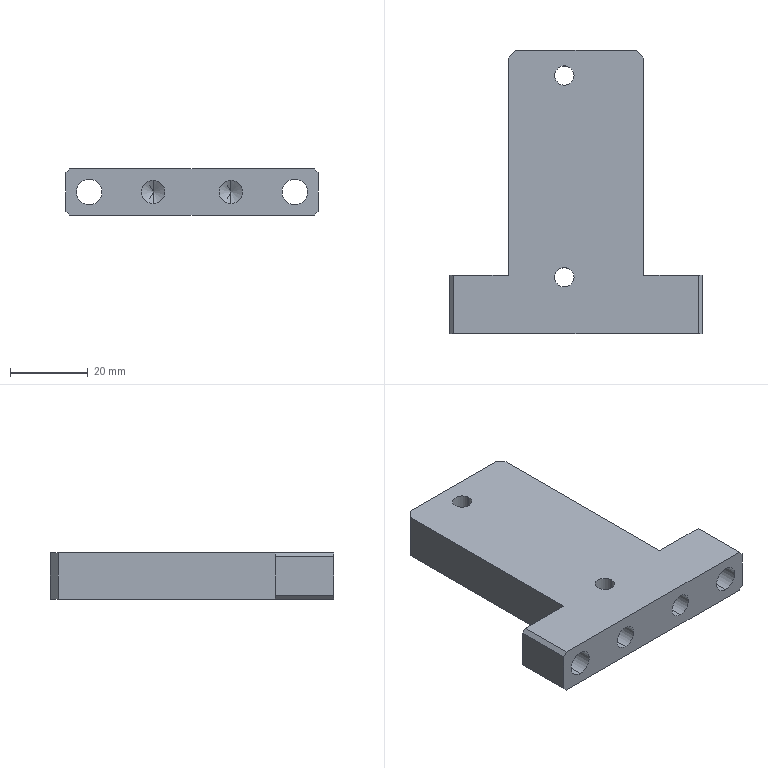Part | SolidWorks | features HoleWzd 3, Chamfer 2, Extrusion 1, ICE 1 | 1 solid | 32 faces | box 65 x 73 x 12 mm | volume 33602 mm3 | plane 16 | cylinder 12 | cone 4 | commonest cylinder face diameters 5 x4 6 x4 6.6 x4
STEP:
#1=CARTESIAN_POINT('',(-0.5,-22.,6.));
#2=VERTEX_POINT('',#1);
#3=CARTESIAN_POINT('',(-5.5,-22.,6.));
#4=VERTEX_POINT('',#3);
#5=CARTESIAN_POINT('',(-3.,-22.,6.));
#6=DIRECTION('',(0.,0.,-1.));
#7=DIRECTION('',(-1.,0.,0.));
#8=AXIS2_PLACEMENT_3D('',#5,#6,#7);
#9=CIRCLE('',#8,2.5);
#10=EDGE_CURVE('',#2,#4,#9,.T.);
#11=ORIENTED_EDGE('',*,*,#10,.F.);
#12=CARTESIAN_POINT('',(-0.5,-22.,-6.));
#13=VERTEX_POINT('',#12);
#14=CARTESIAN_POINT('',(-0.5,-22.,-6.));
#15=DIRECTION('',(0.,0.,-1.));
#16=VECTOR('',#15,1000.);
#17=LINE('',#14,#16);
#18=EDGE_CURVE('',#2,#13,#17,.T.);
#19=ORIENTED_EDGE('',*,*,#18,.T.);
#20=CARTESIAN_POINT('',(-5.5,-22.,-6.));
#21=VERTEX_POINT('',#20);
#22=CARTESIAN_POINT('',(-3.,-22.,-6.));
#23=DIRECTION('',(0.,0.,-1.));
#24=DIRECTION('',(-1.,0.,0.));
#25=AXIS2_PLACEMENT_3D('',#22,#23,#24);
#26=CIRCLE('',#25,2.5);
#27=EDGE_CURVE('',#13,#21,#26,.T.);
#28=ORIENTED_EDGE('',*,*,#27,.T.);
#29=CARTESIAN_POINT('',(-5.5,-22.,-6.));
#30=DIRECTION('',(0.,0.,-1.));
#31=VECTOR('',#30,1000.);
#32=LINE('',#29,#31);
#33=EDGE_CURVE('',#4,#21,#32,.T.);
#34=ORIENTED_EDGE('',*,*,#33,.F.);
#35=EDGE_LOOP('',(#11,#19,#28,#34));
#36=FACE_OUTER_BOUND('',#35,.T.);
#37=CARTESIAN_POINT('',(-3.,-22.,-6.));
#38=DIRECTION('',(0.,0.,-1.));
#39=DIRECTION('',(-1.,0.,0.));
#40=AXIS2_PLACEMENT_3D('',#37,#38,#39);
#41=CYLINDRICAL_SURFACE('',#40,2.5);
#42=ADVANCED_FACE('',(#36),#41,.F.);
#43=CARTESIAN_POINT('',(-0.5,30.,6.));
#44=VERTEX_POINT('',#43);
#45=CARTESIAN_POINT('',(-5.5,30.,6.));
#46=VERTEX_POINT('',#45);
#47=CARTESIAN_POINT('',(-3.,30.,6.));
#48=DIRECTION('',(0.,0.,-1.));
#49=DIRECTION('',(-1.,0.,0.));
#50=AXIS2_PLACEMENT_3D('',#47,#48,#49);
#51=CIRCLE('',#50,2.5);
#52=EDGE_CURVE('',#44,#46,#51,.T.);
#53=ORIENTED_EDGE('',*,*,#52,.F.);
#54=CARTESIAN_POINT('',(-0.5,30.,-6.));
#55=VERTEX_POINT('',#54);
#56=CARTESIAN_POINT('',(-0.5,30.,-6.));
#57=DIRECTION('',(0.,0.,-1.));
#58=VECTOR('',#57,1000.);
#59=LINE('',#56,#58);
#60=EDGE_CURVE('',#44,#55,#59,.T.);
#61=ORIENTED_EDGE('',*,*,#60,.T.);
#62=CARTESIAN_POINT('',(-5.5,30.,-6.));
#63=VERTEX_POINT('',#62);
#64=CARTESIAN_POINT('',(-3.,30.,-6.));
#65=DIRECTION('',(0.,0.,-1.));
#66=DIRECTION('',(-1.,0.,0.));
#67=AXIS2_PLACEMENT_3D('',#64,#65,#66);
#68=CIRCLE('',#67,2.5);
#69=EDGE_CURVE('',#55,#63,#68,.T.);
#70=ORIENTED_EDGE('',*,*,#69,.T.);
#71=CARTESIAN_POINT('',(-5.5,30.,-6.));
#72=DIRECTION('',(0.,0.,-1.));
#73=VECTOR('',#72,1000.);
#74=LINE('',#71,#73);
#75=EDGE_CURVE('',#46,#63,#74,.T.);
#76=ORIENTED_EDGE('',*,*,#75,.F.);
#77=EDGE_LOOP('',(#53,#61,#70,#76));
#78=FACE_OUTER_BOUND('',#77,.T.);
#79=CARTESIAN_POINT('',(-3.,30.,-6.));
#80=DIRECTION('',(0.,0.,-1.));
#81=DIRECTION('',(-1.,0.,0.));
#82=AXIS2_PLACEMENT_3D('',#79,#80,#81);
#83=CYLINDRICAL_SURFACE('',#82,2.5);
#84=ADVANCED_FACE('',(#78),#83,.F.);
#85=CARTESIAN_POINT('',(-10.,-21.5,3.));
#86=VERTEX_POINT('',#85);
#87=CARTESIAN_POINT('',(-10.,-21.5,-3.));
#88=VERTEX_POINT('',#87);
#89=CARTESIAN_POINT('',(-10.,-21.5,0.));
#90=DIRECTION('',(0.,-1.,0.));
#91=DIRECTION('',(0.,0.,-1.));
#92=AXIS2_PLACEMENT_3D('',#89,#90,#91);
#93=CIRCLE('',#92,3.);
#94=EDGE_CURVE('',#86,#88,#93,.T.);
#95=ORIENTED_EDGE('',*,*,#94,.F.);
#96=CARTESIAN_POINT('',(-10.,-36.5,3.));
#97=VERTEX_POINT('',#96);
#98=CARTESIAN_POINT('',(-10.,-36.5,3.));
#99=DIRECTION('',(0.,-1.,0.));
#100=VECTOR('',#99,1000.);
#101=LINE('',#98,#100);
#102=EDGE_CURVE('',#86,#97,#101,.T.);
#103=ORIENTED_EDGE('',*,*,#102,.T.);
#104=CARTESIAN_POINT('',(-10.,-36.5,-3.));
#105=VERTEX_POINT('',#104);
#106=CARTESIAN_POINT('',(-10.,-36.5,0.));
#107=DIRECTION('',(0.,-1.,0.));
#108=DIRECTION('',(0.,0.,-1.));
#109=AXIS2_PLACEMENT_3D('',#106,#107,#108);
#110=CIRCLE('',#109,3.);
#111=EDGE_CURVE('',#97,#105,#110,.T.);
#112=ORIENTED_EDGE('',*,*,#111,.T.);
#113=CARTESIAN_POINT('',(-10.,-36.5,-3.));
#114=DIRECTION('',(0.,-1.,0.));
#115=VECTOR('',#114,1000.);
#116=LINE('',#113,#115);
#117=EDGE_CURVE('',#88,#105,#116,.T.);
#118=ORIENTED_EDGE('',*,*,#117,.F.);
#119=EDGE_LOOP('',(#95,#103,#112,#118));
#120=FACE_OUTER_BOUND('',#119,.T.);
#121=CARTESIAN_POINT('',(-10.,-36.5,0.));
#122=DIRECTION('',(0.,-1.,0.));
#123=DIRECTION('',(0.,0.,-1.));
#124=AXIS2_PLACEMENT_3D('',#121,#122,#123);
#125=CYLINDRICAL_SURFACE('',#124,3.);
#126=ADVANCED_FACE('',(#120),#125,.F.);
#127=CARTESIAN_POINT('',(-10.,-19.697,0.));
#128=VERTEX_POINT('',#127);
#129=CARTESIAN_POINT('',(-10.,-21.5,-3.));
#130=DIRECTION('',(0.,-0.515,-0.8572));
#131=VECTOR('',#130,1000.);
#132=LINE('',#129,#131);
#133=EDGE_CURVE('',#128,#88,#132,.T.);
#134=ORIENTED_EDGE('',*,*,#133,.F.);
#135=CARTESIAN_POINT('',(-10.,-21.5,3.));
#136=DIRECTION('',(0.,-0.515,0.8572));
#137=VECTOR('',#136,1000.);
#138=LINE('',#135,#137);
#139=EDGE_CURVE('',#128,#86,#138,.T.);
#140=ORIENTED_EDGE('',*,*,#139,.T.);
#141=ORIENTED_EDGE('',*,*,#94,.T.);
#142=EDGE_LOOP('',(#134,#140,#141));
#143=FACE_OUTER_BOUND('',#142,.T.);
#144=CARTESIAN_POINT('',(-10.,-21.5,0.));
#145=DIRECTION('',(0.,-1.,0.));
#146=DIRECTION('',(0.,0.,-1.));
#147=AXIS2_PLACEMENT_3D('',#144,#145,#146);
#148=CONICAL_SURFACE('',#147,3.,1.03);
#149=ADVANCED_FACE('',(#143),#148,.F.);
#150=CARTESIAN_POINT('',(10.,-21.5,3.));
#151=VERTEX_POINT('',#150);
#152=CARTESIAN_POINT('',(10.,-21.5,-3.));
#153=VERTEX_POINT('',#152);
#154=CARTESIAN_POINT('',(10.,-21.5,0.));
#155=DIRECTION('',(0.,-1.,0.));
#156=DIRECTION('',(0.,0.,-1.));
#157=AXIS2_PLACEMENT_3D('',#154,#155,#156);
#158=CIRCLE('',#157,3.);
#159=EDGE_CURVE('',#151,#153,#158,.T.);
#160=ORIENTED_EDGE('',*,*,#159,.F.);
#161=CARTESIAN_POINT('',(10.,-36.5,3.));
#162=VERTEX_POINT('',#161);
#163=CARTESIAN_POINT('',(10.,-36.5,3.));
#164=DIRECTION('',(0.,-1.,0.));
#165=VECTOR('',#164,1000.);
#166=LINE('',#163,#165);
#167=EDGE_CURVE('',#151,#162,#166,.T.);
#168=ORIENTED_EDGE('',*,*,#167,.T.);
#169=CARTESIAN_POINT('',(10.,-36.5,-3.));
#170=VERTEX_POINT('',#169);
#171=CARTESIAN_POINT('',(10.,-36.5,0.));
#172=DIRECTION('',(0.,-1.,0.));
#173=DIRECTION('',(0.,0.,-1.));
#174=AXIS2_PLACEMENT_3D('',#171,#172,#173);
#175=CIRCLE('',#174,3.);
#176=EDGE_CURVE('',#162,#170,#175,.T.);
#177=ORIENTED_EDGE('',*,*,#176,.T.);
#178=CARTESIAN_POINT('',(10.,-36.5,-3.));
#179=DIRECTION('',(0.,-1.,0.));
#180=VECTOR('',#179,1000.);
#181=LINE('',#178,#180);
#182=EDGE_CURVE('',#153,#170,#181,.T.);
#183=ORIENTED_EDGE('',*,*,#182,.F.);
#184=EDGE_LOOP('',(#160,#168,#177,#183));
#185=FACE_OUTER_BOUND('',#184,.T.);
#186=CARTESIAN_POINT('',(10.,-36.5,0.));
#187=DIRECTION('',(0.,-1.,0.));
#188=DIRECTION('',(0.,0.,-1.));
#189=AXIS2_PLACEMENT_3D('',#186,#187,#188);
#190=CYLINDRICAL_SURFACE('',#189,3.);
#191=ADVANCED_FACE('',(#185),#190,.F.);
#192=CARTESIAN_POINT('',(10.,-19.697,0.));
#193=VERTEX_POINT('',#192);
#194=CARTESIAN_POINT('',(10.,-21.5,-3.));
#195=DIRECTION('',(0.,-0.515,-0.8572));
#196=VECTOR('',#195,1000.);
#197=LINE('',#194,#196);
#198=EDGE_CURVE('',#193,#153,#197,.T.);
#199=ORIENTED_EDGE('',*,*,#198,.F.);
#200=CARTESIAN_POINT('',(10.,-21.5,3.));
#201=DIRECTION('',(0.,-0.515,0.8572));
#202=VECTOR('',#201,1000.);
#203=LINE('',#200,#202);
#204=EDGE_CURVE('',#193,#151,#203,.T.);
#205=ORIENTED_EDGE('',*,*,#204,.T.);
#206=ORIENTED_EDGE('',*,*,#159,.T.);
#207=EDGE_LOOP('',(#199,#205,#206));
#208=FACE_OUTER_BOUND('',#207,.T.);
#209=CARTESIAN_POINT('',(10.,-21.5,0.));
#210=DIRECTION('',(0.,-1.,0.));
#211=DIRECTION('',(0.,0.,-1.));
#212=AXIS2_PLACEMENT_3D('',#209,#210,#211);
#213=CONICAL_SURFACE('',#212,3.,1.03);
#214=ADVANCED_FACE('',(#208),#213,.F.);
#215=CARTESIAN_POINT('',(-26.5,-36.5,-3.3));
#216=VERTEX_POINT('',#215);
#217=CARTESIAN_POINT('',(-26.5,-36.5,3.3));
#218=VERTEX_POINT('',#217);
#219=CARTESIAN_POINT('',(-26.5,-36.5,0.));
#220=DIRECTION('',(0.,1.,0.));
#221=DIRECTION('',(0.,0.,1.));
#222=AXIS2_PLACEMENT_3D('',#219,#220,#221);
#223=CIRCLE('',#222,3.3);
#224=EDGE_CURVE('',#216,#218,#223,.T.);
#225=ORIENTED_EDGE('',*,*,#224,.F.);
#226=CARTESIAN_POINT('',(-26.5,-21.5,-3.3));
#227=VERTEX_POINT('',#226);
#228=CARTESIAN_POINT('',(-26.5,-21.5,-3.3));
#229=DIRECTION('',(0.,1.,0.));
#230=VECTOR('',#229,1000.);
#231=LINE('',#228,#230);
#232=EDGE_CURVE('',#216,#227,#231,.T.);
#233=ORIENTED_EDGE('',*,*,#232,.T.);
#234=CARTESIAN_POINT('',(-26.5,-21.5,3.3));
#235=VERTEX_POINT('',#234);
#236=CARTESIAN_POINT('',(-26.5,-21.5,0.));
#237=DIRECTION('',(0.,1.,0.));
#238=DIRECTION('',(0.,0.,1.));
#239=AXIS2_PLACEMENT_3D('',#236,#237,#238);
#240=CIRCLE('',#239,3.3);
#241=EDGE_CURVE('',#227,#235,#240,.T.);
#242=ORIENTED_EDGE('',*,*,#241,.T.);
#243=CARTESIAN_POINT('',(-26.5,-21.5,3.3));
#244=DIRECTION('',(0.,1.,0.));
#245=VECTOR('',#244,1000.);
#246=LINE('',#243,#245);
#247=EDGE_CURVE('',#218,#235,#246,.T.);
#248=ORIENTED_EDGE('',*,*,#247,.F.);
#249=EDGE_LOOP('',(#225,#233,#242,#248));
#250=FACE_OUTER_BOUND('',#249,.T.);
#251=CARTESIAN_POINT('',(-26.5,-21.5,0.));
#252=DIRECTION('',(0.,1.,0.));
#253=DIRECTION('',(0.,0.,1.));
#254=AXIS2_PLACEMENT_3D('',#251,#252,#253);
#255=CYLINDRICAL_SURFACE('',#254,3.3);
#256=ADVANCED_FACE('',(#250),#255,.F.);
#257=CARTESIAN_POINT('',(26.5,-36.5,-3.3));
#258=VERTEX_POINT('',#257);
#259=CARTESIAN_POINT('',(26.5,-36.5,3.3));
#260=VERTEX_POINT('',#259);
#261=CARTESIAN_POINT('',(26.5,-36.5,0.));
#262=DIRECTION('',(0.,1.,0.));
#263=DIRECTION('',(0.,0.,1.));
#264=AXIS2_PLACEMENT_3D('',#261,#262,#263);
#265=CIRCLE('',#264,3.3);
#266=EDGE_CURVE('',#258,#260,#265,.T.);
#267=ORIENTED_EDGE('',*,*,#266,.F.);
#268=CARTESIAN_POINT('',(26.5,-21.5,-3.3));
#269=VERTEX_POINT('',#268);
#270=CARTESIAN_POINT('',(26.5,-21.5,-3.3));
#271=DIRECTION('',(0.,1.,0.));
#272=VECTOR('',#271,1000.);
#273=LINE('',#270,#272);
#274=EDGE_CURVE('',#258,#269,#273,.T.);
#275=ORIENTED_EDGE('',*,*,#274,.T.);
#276=CARTESIAN_POINT('',(26.5,-21.5,3.3));
#277=VERTEX_POINT('',#276);
#278=CARTESIAN_POINT('',(26.5,-21.5,0.));
#279=DIRECTION('',(0.,1.,0.));
#280=DIRECTION('',(0.,0.,1.));
#281=AXIS2_PLACEMENT_3D('',#278,#279,#280);
#282=CIRCLE('',#281,3.3);
#283=EDGE_CURVE('',#269,#277,#282,.T.);
#284=ORIENTED_EDGE('',*,*,#283,.T.);
#285=CARTESIAN_POINT('',(26.5,-21.5,3.3));
#286=DIRECTION('',(0.,1.,0.));
#287=VECTOR('',#286,1000.);
#288=LINE('',#285,#287);
#289=EDGE_CURVE('',#260,#277,#288,.T.);
#290=ORIENTED_EDGE('',*,*,#289,.F.);
#291=EDGE_LOOP('',(#267,#275,#284,#290));
#292=FACE_OUTER_BOUND('',#291,.T.);
#293=CARTESIAN_POINT('',(26.5,-21.5,0.));
#294=DIRECTION('',(0.,1.,0.));
#295=DIRECTION('',(0.,0.,1.));
#296=AXIS2_PLACEMENT_3D('',#293,#294,#295);
#297=CYLINDRICAL_SURFACE('',#296,3.3);
#298=ADVANCED_FACE('',(#292),#297,.F.);
#299=CARTESIAN_POINT('',(17.5,-21.5,-6.));
#300=VERTEX_POINT('',#299);
#301=CARTESIAN_POINT('',(17.5,34.5,-6.));
#302=VERTEX_POINT('',#301);
#303=CARTESIAN_POINT('',(17.5,-36.5,-6.));
#304=DIRECTION('',(0.,1.,0.));
#305=VECTOR('',#304,1000.);
#306=LINE('',#303,#305);
#307=EDGE_CURVE('',#300,#302,#306,.T.);
#308=ORIENTED_EDGE('',*,*,#307,.T.);
#309=CARTESIAN_POINT('',(17.5,34.5,6.));
#310=VERTEX_POINT('',#309);
#311=CARTESIAN_POINT('',(17.5,34.5,6.));
#312=DIRECTION('',(0.,0.,1.));
#313=VECTOR('',#312,1000.);
#314=LINE('',#311,#313);
#315=EDGE_CURVE('',#302,#310,#314,.T.);
#316=ORIENTED_EDGE('',*,*,#315,.T.);
#317=CARTESIAN_POINT('',(17.5,-21.5,6.));
#318=VERTEX_POINT('',#317);
#319=CARTESIAN_POINT('',(17.5,-36.5,6.));
#320=DIRECTION('',(0.,1.,0.));
#321=VECTOR('',#320,1000.);
#322=LINE('',#319,#321);
#323=EDGE_CURVE('',#318,#310,#322,.T.);
#324=ORIENTED_EDGE('',*,*,#323,.F.);
#325=CARTESIAN_POINT('',(17.5,-21.5,6.));
#326=DIRECTION('',(0.,0.,1.));
#327=VECTOR('',#326,1000.);
#328=LINE('',#325,#327);
#329=EDGE_CURVE('',#300,#318,#328,.T.);
#330=ORIENTED_EDGE('',*,*,#329,.F.);
#331=EDGE_LOOP('',(#308,#316,#324,#330));
#332=FACE_OUTER_BOUND('',#331,.T.);
#333=CARTESIAN_POINT('',(17.5,-36.5,6.));
#334=DIRECTION('',(-1.,0.,0.));
#335=DIRECTION('',(0.,0.,1.));
#336=AXIS2_PLACEMENT_3D('',#333,#334,#335);
#337=PLANE('',#336);
#338=ADVANCED_FACE('',(#332),#337,.F.);
#339=CARTESIAN_POINT('',(-17.5,34.5,6.));
#340=VERTEX_POINT('',#339);
#341=CARTESIAN_POINT('',(-17.5,-21.5,6.));
#342=VERTEX_POINT('',#341);
#343=CARTESIAN_POINT('',(-17.5,-36.5,6.));
#344=DIRECTION('',(0.,-1.,0.));
#345=VECTOR('',#344,1000.);
#346=LINE('',#343,#345);
#347=EDGE_CURVE('',#340,#342,#346,.T.);
#348=ORIENTED_EDGE('',*,*,#347,.F.);
#349=CARTESIAN_POINT('',(-17.5,34.5,-6.));
#350=VERTEX_POINT('',#349);
#351=CARTESIAN_POINT('',(-17.5,34.5,6.));
#352=DIRECTION('',(0.,0.,-1.));
#353=VECTOR('',#352,1000.);
#354=LINE('',#351,#353);
#355=EDGE_CURVE('',#340,#350,#354,.T.);
#356=ORIENTED_EDGE('',*,*,#355,.T.);
#357=CARTESIAN_POINT('',(-17.5,-21.5,-6.));
#358=VERTEX_POINT('',#357);
#359=CARTESIAN_POINT('',(-17.5,-36.5,-6.));
#360=DIRECTION('',(0.,-1.,0.));
#361=VECTOR('',#360,1000.);
#362=LINE('',#359,#361);
#363=EDGE_CURVE('',#350,#358,#362,.T.);
#364=ORIENTED_EDGE('',*,*,#363,.T.);
#365=CARTESIAN_POINT('',(-17.5,-21.5,6.));
#366=DIRECTION('',(0.,0.,-1.));
#367=VECTOR('',#366,1000.);
#368=LINE('',#365,#367);
#369=EDGE_CURVE('',#342,#358,#368,.T.);
#370=ORIENTED_EDGE('',*,*,#369,.F.);
#371=EDGE_LOOP('',(#348,#356,#364,#370));
#372=FACE_OUTER_BOUND('',#371,.T.);
#373=CARTESIAN_POINT('',(-17.5,-36.5,6.));
#374=DIRECTION('',(1.,0.,0.));
#375=DIRECTION('',(0.,0.,-1.));
#376=AXIS2_PLACEMENT_3D('',#373,#374,#375);
#377=PLANE('',#376);
#378=ADVANCED_FACE('',(#372),#377,.F.);
#379=CARTESIAN_POINT('',(15.5,36.5,6.));
#380=VERTEX_POINT('',#379);
#381=CARTESIAN_POINT('',(-15.5,36.5,6.));
#382=VERTEX_POINT('',#381);
#383=CARTESIAN_POINT('',(-17.5,36.5,6.));
#384=DIRECTION('',(-1.,0.,0.));
#385=VECTOR('',#384,1000.);
#386=LINE('',#383,#385);
#387=EDGE_CURVE('',#380,#382,#386,.T.);
#388=ORIENTED_EDGE('',*,*,#387,.F.);
#389=CARTESIAN_POINT('',(15.5,36.5,-6.));
#390=VERTEX_POINT('',#389);
#391=CARTESIAN_POINT('',(15.5,36.5,6.));
#392=DIRECTION('',(0.,0.,-1.));
#393=VECTOR('',#392,1000.);
#394=LINE('',#391,#393);
#395=EDGE_CURVE('',#380,#390,#394,.T.);
#396=ORIENTED_EDGE('',*,*,#395,.T.);
#397=CARTESIAN_POINT('',(-15.5,36.5,-6.));
#398=VERTEX_POINT('',#397);
#399=CARTESIAN_POINT('',(-17.5,36.5,-6.));
#400=DIRECTION('',(-1.,0.,0.));
#401=VECTOR('',#400,1000.);
#402=LINE('',#399,#401);
#403=EDGE_CURVE('',#390,#398,#402,.T.);
#404=ORIENTED_EDGE('',*,*,#403,.T.);
#405=CARTESIAN_POINT('',(-15.5,36.5,6.));
#406=DIRECTION('',(0.,0.,1.));
#407=VECTOR('',#406,1000.);
#408=LINE('',#405,#407);
#409=EDGE_CURVE('',#398,#382,#408,.T.);
#410=ORIENTED_EDGE('',*,*,#409,.T.);
#411=EDGE_LOOP('',(#388,#396,#404,#410));
#412=FACE_OUTER_BOUND('',#411,.T.);
#413=CARTESIAN_POINT('',(-17.5,36.5,6.));
#414=DIRECTION('',(0.,-1.,0.));
#415=DIRECTION('',(0.,0.,-1.));
#416=AXIS2_PLACEMENT_3D('',#413,#414,#415);
#417=PLANE('',#416);
#418=ADVANCED_FACE('',(#412),#417,.F.);
#419=CARTESIAN_POINT('',(-10.,-36.5,0.));
#420=DIRECTION('',(0.,-1.,0.));
#421=DIRECTION('',(0.,0.,-1.));
#422=AXIS2_PLACEMENT_3D('',#419,#420,#421);
#423=CIRCLE('',#422,3.);
#424=EDGE_CURVE('',#105,#97,#423,.T.);
#425=ORIENTED_EDGE('',*,*,#424,.F.);
#426=ORIENTED_EDGE('',*,*,#111,.F.);
#427=EDGE_LOOP('',(#425,#426));
#428=FACE_BOUND('',#427,.T.);
#429=CARTESIAN_POINT('',(10.,-36.5,0.));
#430=DIRECTION('',(0.,-1.,0.));
#431=DIRECTION('',(0.,0.,-1.));
#432=AXIS2_PLACEMENT_3D('',#429,#430,#431);
#433=CIRCLE('',#432,3.);
#434=EDGE_CURVE('',#170,#162,#433,.T.);
#435=ORIENTED_EDGE('',*,*,#434,.F.);
#436=ORIENTED_EDGE('',*,*,#176,.F.);
#437=EDGE_LOOP('',(#435,#436));
#438=FACE_BOUND('',#437,.T.);
#439=CARTESIAN_POINT('',(-26.5,-36.5,0.));
#440=DIRECTION('',(0.,1.,0.));
#441=DIRECTION('',(0.,0.,1.));
#442=AXIS2_PLACEMENT_3D('',#439,#440,#441);
#443=CIRCLE('',#442,3.3);
#444=EDGE_CURVE('',#218,#216,#443,.T.);
#445=ORIENTED_EDGE('',*,*,#444,.T.);
#446=ORIENTED_EDGE('',*,*,#224,.T.);
#447=EDGE_LOOP('',(#445,#446));
#448=FACE_BOUND('',#447,.T.);
#449=CARTESIAN_POINT('',(26.5,-36.5,0.));
#450=DIRECTION('',(0.,1.,0.));
#451=DIRECTION('',(0.,0.,1.));
#452=AXIS2_PLACEMENT_3D('',#449,#450,#451);
#453=CIRCLE('',#452,3.3);
#454=EDGE_CURVE('',#260,#258,#453,.T.);
#455=ORIENTED_EDGE('',*,*,#454,.T.);
#456=ORIENTED_EDGE('',*,*,#266,.T.);
#457=EDGE_LOOP('',(#455,#456));
#458=FACE_BOUND('',#457,.T.);
#459=CARTESIAN_POINT('',(-31.5,-36.5,-6.));
#460=VERTEX_POINT('',#459);
#461=CARTESIAN_POINT('',(31.5,-36.5,-6.));
#462=VERTEX_POINT('',#461);
#463=CARTESIAN_POINT('',(-17.5,-36.5,-6.));
#464=DIRECTION('',(1.,0.,0.));
#465=VECTOR('',#464,1000.);
#466=LINE('',#463,#465);
#467=EDGE_CURVE('',#460,#462,#466,.T.);
#468=ORIENTED_EDGE('',*,*,#467,.T.);
#469=CARTESIAN_POINT('',(32.5,-36.5,-5.));
#470=VERTEX_POINT('',#469);
#471=CARTESIAN_POINT('',(31.5,-36.5,-6.));
#472=DIRECTION('',(0.7071,0.,0.7071));
#473=VECTOR('',#472,1000.);
#474=LINE('',#471,#473);
#475=EDGE_CURVE('',#462,#470,#474,.T.);
#476=ORIENTED_EDGE('',*,*,#475,.T.);
#477=CARTESIAN_POINT('',(32.5,-36.5,5.));
#478=VERTEX_POINT('',#477);
#479=CARTESIAN_POINT('',(32.5,-36.5,-6.));
#480=DIRECTION('',(0.,0.,1.));
#481=VECTOR('',#480,1000.);
#482=LINE('',#479,#481);
#483=EDGE_CURVE('',#470,#478,#482,.T.);
#484=ORIENTED_EDGE('',*,*,#483,.T.);
#485=CARTESIAN_POINT('',(31.5,-36.5,6.));
#486=VERTEX_POINT('',#485);
#487=CARTESIAN_POINT('',(32.5,-36.5,5.));
#488=DIRECTION('',(-0.7071,0.,0.7071));
#489=VECTOR('',#488,1000.);
#490=LINE('',#487,#489);
#491=EDGE_CURVE('',#478,#486,#490,.T.);
#492=ORIENTED_EDGE('',*,*,#491,.T.);
#493=CARTESIAN_POINT('',(-31.5,-36.5,6.));
#494=VERTEX_POINT('',#493);
#495=CARTESIAN_POINT('',(-17.5,-36.5,6.));
#496=DIRECTION('',(1.,0.,0.));
#497=VECTOR('',#496,1000.);
#498=LINE('',#495,#497);
#499=EDGE_CURVE('',#494,#486,#498,.T.);
#500=ORIENTED_EDGE('',*,*,#499,.F.);
#501=CARTESIAN_POINT('',(-32.5,-36.5,5.));
#502=VERTEX_POINT('',#501);
#503=CARTESIAN_POINT('',(-31.5,-36.5,6.));
#504=DIRECTION('',(-0.7071,0.,-0.7071));
#505=VECTOR('',#504,1000.);
#506=LINE('',#503,#505);
#507=EDGE_CURVE('',#494,#502,#506,.T.);
#508=ORIENTED_EDGE('',*,*,#507,.T.);
#509=CARTESIAN_POINT('',(-32.5,-36.5,-5.));
#510=VERTEX_POINT('',#509);
#511=CARTESIAN_POINT('',(-32.5,-36.5,-6.));
#512=DIRECTION('',(0.,0.,-1.));
#513=VECTOR('',#512,1000.);
#514=LINE('',#511,#513);
#515=EDGE_CURVE('',#502,#510,#514,.T.);
#516=ORIENTED_EDGE('',*,*,#515,.T.);
#517=CARTESIAN_POINT('',(-32.5,-36.5,-5.));
#518=DIRECTION('',(0.7071,0.,-0.7071));
#519=VECTOR('',#518,1000.);
#520=LINE('',#517,#519);
#521=EDGE_CURVE('',#510,#460,#520,.T.);
#522=ORIENTED_EDGE('',*,*,#521,.T.);
#523=EDGE_LOOP('',(#468,#476,#484,#492,#500,#508,#516,#522));
#524=FACE_OUTER_BOUND('',#523,.T.);
#525=CARTESIAN_POINT('',(-17.5,-36.5,6.));
#526=DIRECTION('',(0.,1.,0.));
#527=DIRECTION('',(0.,0.,1.));
#528=AXIS2_PLACEMENT_3D('',#525,#526,#527);
#529=PLANE('',#528);
#530=ADVANCED_FACE('',(#428,#438,#448,#458,#524),#529,.F.);
#531=CARTESIAN_POINT('',(-3.,-22.,6.));
#532=DIRECTION('',(0.,0.,-1.));
#533=DIRECTION('',(-1.,0.,0.));
#534=AXIS2_PLACEMENT_3D('',#531,#532,#533);
#535=CIRCLE('',#534,2.5);
#536=EDGE_CURVE('',#4,#2,#535,.T.);
#537=ORIENTED_EDGE('',*,*,#536,.T.);
#538=ORIENTED_EDGE('',*,*,#10,.T.);
#539=EDGE_LOOP('',(#537,#538));
#540=FACE_BOUND('',#539,.T.);
#541=CARTESIAN_POINT('',(-3.,30.,6.));
#542=DIRECTION('',(0.,0.,-1.));
#543=DIRECTION('',(-1.,0.,0.));
#544=AXIS2_PLACEMENT_3D('',#541,#542,#543);
#545=CIRCLE('',#544,2.5);
#546=EDGE_CURVE('',#46,#44,#545,.T.);
#547=ORIENTED_EDGE('',*,*,#546,.T.);
#548=ORIENTED_EDGE('',*,*,#52,.T.);
#549=EDGE_LOOP('',(#547,#548));
#550=FACE_BOUND('',#549,.T.);
#551=ORIENTED_EDGE('',*,*,#323,.T.);
#552=CARTESIAN_POINT('',(15.5,36.5,6.));
#553=DIRECTION('',(-0.7071,0.7071,0.));
#554=VECTOR('',#553,1000.);
#555=LINE('',#552,#554);
#556=EDGE_CURVE('',#310,#380,#555,.T.);
#557=ORIENTED_EDGE('',*,*,#556,.T.);
#558=ORIENTED_EDGE('',*,*,#387,.T.);
#559=CARTESIAN_POINT('',(-17.5,34.5,6.));
#560=DIRECTION('',(-0.7071,-0.7071,0.));
#561=VECTOR('',#560,1000.);
#562=LINE('',#559,#561);
#563=EDGE_CURVE('',#382,#340,#562,.T.);
#564=ORIENTED_EDGE('',*,*,#563,.T.);
#565=ORIENTED_EDGE('',*,*,#347,.T.);
#566=CARTESIAN_POINT('',(-31.5,-21.5,6.));
#567=VERTEX_POINT('',#566);
#568=CARTESIAN_POINT('',(32.5,-21.5,6.));
#569=DIRECTION('',(-1.,0.,0.));
#570=VECTOR('',#569,1000.);
#571=LINE('',#568,#570);
#572=EDGE_CURVE('',#342,#567,#571,.T.);
#573=ORIENTED_EDGE('',*,*,#572,.T.);
#574=CARTESIAN_POINT('',(-31.5,-36.5,6.));
#575=DIRECTION('',(0.,-1.,0.));
#576=VECTOR('',#575,1000.);
#577=LINE('',#574,#576);
#578=EDGE_CURVE('',#567,#494,#577,.T.);
#579=ORIENTED_EDGE('',*,*,#578,.T.);
#580=ORIENTED_EDGE('',*,*,#499,.T.);
#581=CARTESIAN_POINT('',(31.5,-21.5,6.));
#582=VERTEX_POINT('',#581);
#583=CARTESIAN_POINT('',(31.5,-21.5,6.));
#584=DIRECTION('',(0.,1.,0.));
#585=VECTOR('',#584,1000.);
#586=LINE('',#583,#585);
#587=EDGE_CURVE('',#486,#582,#586,.T.);
#588=ORIENTED_EDGE('',*,*,#587,.T.);
#589=CARTESIAN_POINT('',(32.5,-21.5,6.));
#590=DIRECTION('',(-1.,0.,0.));
#591=VECTOR('',#590,1000.);
#592=LINE('',#589,#591);
#593=EDGE_CURVE('',#582,#318,#592,.T.);
#594=ORIENTED_EDGE('',*,*,#593,.T.);
#595=EDGE_LOOP('',(#551,#557,#558,#564,#565,#573,#579,#580,#588,#594));
#596=FACE_OUTER_BOUND('',#595,.T.);
#597=CARTESIAN_POINT('',(0.,0.,6.));
#598=DIRECTION('',(0.,0.,-1.));
#599=DIRECTION('',(-1.,0.,0.));
#600=AXIS2_PLACEMENT_3D('',#597,#598,#599);
#601=PLANE('',#600);
#602=ADVANCED_FACE('',(#540,#550,#596),#601,.F.);
#603=CARTESIAN_POINT('',(-3.,-22.,-6.));
#604=DIRECTION('',(0.,0.,-1.));
#605=DIRECTION('',(-1.,0.,0.));
#606=AXIS2_PLACEMENT_3D('',#603,#604,#605);
#607=CIRCLE('',#606,2.5);
#608=EDGE_CURVE('',#21,#13,#607,.T.);
#609=ORIENTED_EDGE('',*,*,#608,.F.);
#610=ORIENTED_EDGE('',*,*,#27,.F.);
#611=EDGE_LOOP('',(#609,#610));
#612=FACE_BOUND('',#611,.T.);
#613=CARTESIAN_POINT('',(-3.,30.,-6.));
#614=DIRECTION('',(0.,0.,-1.));
#615=DIRECTION('',(-1.,0.,0.));
#616=AXIS2_PLACEMENT_3D('',#613,#614,#615);
#617=CIRCLE('',#616,2.5);
#618=EDGE_CURVE('',#63,#55,#617,.T.);
#619=ORIENTED_EDGE('',*,*,#618,.F.);
#620=ORIENTED_EDGE('',*,*,#69,.F.);
#621=EDGE_LOOP('',(#619,#620));
#622=FACE_BOUND('',#621,.T.);
#623=ORIENTED_EDGE('',*,*,#403,.F.);
#624=CARTESIAN_POINT('',(26.,26.,-6.));
#625=DIRECTION('',(0.7071,-0.7071,0.));
#626=VECTOR('',#625,1000.);
#627=LINE('',#624,#626);
#628=EDGE_CURVE('',#390,#302,#627,.T.);
#629=ORIENTED_EDGE('',*,*,#628,.T.);
#630=ORIENTED_EDGE('',*,*,#307,.F.);
#631=CARTESIAN_POINT('',(31.5,-21.5,-6.));
#632=VERTEX_POINT('',#631);
#633=CARTESIAN_POINT('',(32.5,-21.5,-6.));
#634=DIRECTION('',(1.,0.,0.));
#635=VECTOR('',#634,1000.);
#636=LINE('',#633,#635);
#637=EDGE_CURVE('',#300,#632,#636,.T.);
#638=ORIENTED_EDGE('',*,*,#637,.T.);
#639=CARTESIAN_POINT('',(31.5,0.,-6.));
#640=DIRECTION('',(0.,-1.,0.));
#641=VECTOR('',#640,1000.);
#642=LINE('',#639,#641);
#643=EDGE_CURVE('',#632,#462,#642,.T.);
#644=ORIENTED_EDGE('',*,*,#643,.T.);
#645=ORIENTED_EDGE('',*,*,#467,.F.);
#646=CARTESIAN_POINT('',(-31.5,-21.5,-6.));
#647=VERTEX_POINT('',#646);
#648=CARTESIAN_POINT('',(-31.5,0.,-6.));
#649=DIRECTION('',(0.,1.,0.));
#650=VECTOR('',#649,1000.);
#651=LINE('',#648,#650);
#652=EDGE_CURVE('',#460,#647,#651,.T.);
#653=ORIENTED_EDGE('',*,*,#652,.T.);
#654=CARTESIAN_POINT('',(32.5,-21.5,-6.));
#655=DIRECTION('',(1.,0.,0.));
#656=VECTOR('',#655,1000.);
#657=LINE('',#654,#656);
#658=EDGE_CURVE('',#647,#358,#657,.T.);
#659=ORIENTED_EDGE('',*,*,#658,.T.);
#660=ORIENTED_EDGE('',*,*,#363,.F.);
#661=CARTESIAN_POINT('',(-26.,26.,-6.));
#662=DIRECTION('',(0.7071,0.7071,0.));
#663=VECTOR('',#662,1000.);
#664=LINE('',#661,#663);
#665=EDGE_CURVE('',#350,#398,#664,.T.);
#666=ORIENTED_EDGE('',*,*,#665,.T.);
#667=EDGE_LOOP('',(#623,#629,#630,#638,#644,#645,#653,#659,#660,#666));
#668=FACE_OUTER_BOUND('',#667,.T.);
#669=CARTESIAN_POINT('',(0.,0.,-6.));
#670=DIRECTION('',(0.,0.,-1.));
#671=DIRECTION('',(-1.,0.,0.));
#672=AXIS2_PLACEMENT_3D('',#669,#670,#671);
#673=PLANE('',#672);
#674=ADVANCED_FACE('',(#612,#622,#668),#673,.T.);
#675=ORIENTED_EDGE('',*,*,#515,.F.);
#676=CARTESIAN_POINT('',(-32.5,-21.5,5.));
#677=VERTEX_POINT('',#676);
#678=CARTESIAN_POINT('',(-32.5,-21.5,5.));
#679=DIRECTION('',(0.,1.,0.));
#680=VECTOR('',#679,1000.);
#681=LINE('',#678,#680);
#682=EDGE_CURVE('',#502,#677,#681,.T.);
#683=ORIENTED_EDGE('',*,*,#682,.T.);
#684=CARTESIAN_POINT('',(-32.5,-21.5,-5.));
#685=VERTEX_POINT('',#684);
#686=CARTESIAN_POINT('',(-32.5,-21.5,-6.));
#687=DIRECTION('',(0.,0.,-1.));
#688=VECTOR('',#687,1000.);
#689=LINE('',#686,#688);
#690=EDGE_CURVE('',#677,#685,#689,.T.);
#691=ORIENTED_EDGE('',*,*,#690,.T.);
#692=CARTESIAN_POINT('',(-32.5,-21.5,-5.));
#693=DIRECTION('',(0.,-1.,0.));
#694=VECTOR('',#693,1000.);
#695=LINE('',#692,#694);
#696=EDGE_CURVE('',#685,#510,#695,.T.);
#697=ORIENTED_EDGE('',*,*,#696,.T.);
#698=EDGE_LOOP('',(#675,#683,#691,#697));
#699=FACE_OUTER_BOUND('',#698,.T.);
#700=CARTESIAN_POINT('',(-32.5,-21.5,-6.));
#701=DIRECTION('',(-1.,0.,0.));
#702=DIRECTION('',(0.,0.,1.));
#703=AXIS2_PLACEMENT_3D('',#700,#701,#702);
#704=PLANE('',#703);
#705=ADVANCED_FACE('',(#699),#704,.T.);
#706=CARTESIAN_POINT('',(-26.5,-21.5,0.));
#707=DIRECTION('',(0.,1.,0.));
#708=DIRECTION('',(0.,0.,1.));
#709=AXIS2_PLACEMENT_3D('',#706,#707,#708);
#710=CIRCLE('',#709,3.3);
#711=EDGE_CURVE('',#235,#227,#710,.T.);
#712=ORIENTED_EDGE('',*,*,#711,.F.);
#713=ORIENTED_EDGE('',*,*,#241,.F.);
#714=EDGE_LOOP('',(#712,#713));
#715=FACE_BOUND('',#714,.T.);
#716=ORIENTED_EDGE('',*,*,#690,.F.);
#717=CARTESIAN_POINT('',(-31.5,-21.5,6.));
#718=DIRECTION('',(0.7071,0.,0.7071));
#719=VECTOR('',#718,1000.);
#720=LINE('',#717,#719);
#721=EDGE_CURVE('',#677,#567,#720,.T.);
#722=ORIENTED_EDGE('',*,*,#721,.T.);
#723=ORIENTED_EDGE('',*,*,#572,.F.);
#724=ORIENTED_EDGE('',*,*,#369,.T.);
#725=ORIENTED_EDGE('',*,*,#658,.F.);
#726=CARTESIAN_POINT('',(-32.5,-21.5,-5.));
#727=DIRECTION('',(-0.7071,0.,0.7071));
#728=VECTOR('',#727,1000.);
#729=LINE('',#726,#728);
#730=EDGE_CURVE('',#647,#685,#729,.T.);
#731=ORIENTED_EDGE('',*,*,#730,.T.);
#732=EDGE_LOOP('',(#716,#722,#723,#724,#725,#731));
#733=FACE_OUTER_BOUND('',#732,.T.);
#734=CARTESIAN_POINT('',(0.,-21.5,0.));
#735=DIRECTION('',(0.,-1.,0.));
#736=DIRECTION('',(0.,0.,-1.));
#737=AXIS2_PLACEMENT_3D('',#734,#735,#736);
#738=PLANE('',#737);
#739=ADVANCED_FACE('',(#715,#733),#738,.F.);
#740=CARTESIAN_POINT('',(26.5,-21.5,0.));
#741=DIRECTION('',(0.,1.,0.));
#742=DIRECTION('',(0.,0.,1.));
#743=AXIS2_PLACEMENT_3D('',#740,#741,#742);
#744=CIRCLE('',#743,3.3);
#745=EDGE_CURVE('',#277,#269,#744,.T.);
#746=ORIENTED_EDGE('',*,*,#745,.F.);
#747=ORIENTED_EDGE('',*,*,#283,.F.);
#748=EDGE_LOOP('',(#746,#747));
#749=FACE_BOUND('',#748,.T.);
#750=CARTESIAN_POINT('',(32.5,-21.5,-5.));
#751=VERTEX_POINT('',#750);
#752=CARTESIAN_POINT('',(32.5,-21.5,5.));
#753=VERTEX_POINT('',#752);
#754=CARTESIAN_POINT('',(32.5,-21.5,-6.));
#755=DIRECTION('',(0.,0.,1.));
#756=VECTOR('',#755,1000.);
#757=LINE('',#754,#756);
#758=EDGE_CURVE('',#751,#753,#757,.T.);
#759=ORIENTED_EDGE('',*,*,#758,.F.);
#760=CARTESIAN_POINT('',(31.5,-21.5,-6.));
#761=DIRECTION('',(-0.7071,0.,-0.7071));
#762=VECTOR('',#761,1000.);
#763=LINE('',#760,#762);
#764=EDGE_CURVE('',#751,#632,#763,.T.);
#765=ORIENTED_EDGE('',*,*,#764,.T.);
#766=ORIENTED_EDGE('',*,*,#637,.F.);
#767=ORIENTED_EDGE('',*,*,#329,.T.);
#768=ORIENTED_EDGE('',*,*,#593,.F.);
#769=CARTESIAN_POINT('',(32.5,-21.5,5.));
#770=DIRECTION('',(0.7071,0.,-0.7071));
#771=VECTOR('',#770,1000.);
#772=LINE('',#769,#771);
#773=EDGE_CURVE('',#582,#753,#772,.T.);
#774=ORIENTED_EDGE('',*,*,#773,.T.);
#775=EDGE_LOOP('',(#759,#765,#766,#767,#768,#774));
#776=FACE_OUTER_BOUND('',#775,.T.);
#777=CARTESIAN_POINT('',(0.,-21.5,0.));
#778=DIRECTION('',(0.,-1.,0.));
#779=DIRECTION('',(0.,0.,-1.));
#780=AXIS2_PLACEMENT_3D('',#777,#778,#779);
#781=PLANE('',#780);
#782=ADVANCED_FACE('',(#749,#776),#781,.F.);
#783=ORIENTED_EDGE('',*,*,#483,.F.);
#784=CARTESIAN_POINT('',(32.5,-21.5,-5.));
#785=DIRECTION('',(0.,1.,0.));
#786=VECTOR('',#785,1000.);
#787=LINE('',#784,#786);
#788=EDGE_CURVE('',#470,#751,#787,.T.);
#789=ORIENTED_EDGE('',*,*,#788,.T.);
#790=ORIENTED_EDGE('',*,*,#758,.T.);
#791=CARTESIAN_POINT('',(32.5,-36.5,5.));
#792=DIRECTION('',(0.,-1.,0.));
#793=VECTOR('',#792,1000.);
#794=LINE('',#791,#793);
#795=EDGE_CURVE('',#753,#478,#794,.T.);
#796=ORIENTED_EDGE('',*,*,#795,.T.);
#797=EDGE_LOOP('',(#783,#789,#790,#796));
#798=FACE_OUTER_BOUND('',#797,.T.);
#799=CARTESIAN_POINT('',(32.5,-21.5,-6.));
#800=DIRECTION('',(1.,0.,0.));
#801=DIRECTION('',(0.,0.,-1.));
#802=AXIS2_PLACEMENT_3D('',#799,#800,#801);
#803=PLANE('',#802);
#804=ADVANCED_FACE('',(#798),#803,.T.);
#805=ORIENTED_EDGE('',*,*,#274,.F.);
#806=ORIENTED_EDGE('',*,*,#454,.F.);
#807=ORIENTED_EDGE('',*,*,#289,.T.);
#808=ORIENTED_EDGE('',*,*,#745,.T.);
#809=EDGE_LOOP('',(#805,#806,#807,#808));
#810=FACE_OUTER_BOUND('',#809,.T.);
#811=CARTESIAN_POINT('',(26.5,-21.5,0.));
#812=DIRECTION('',(0.,1.,0.));
#813=DIRECTION('',(0.,0.,1.));
#814=AXIS2_PLACEMENT_3D('',#811,#812,#813);
#815=CYLINDRICAL_SURFACE('',#814,3.3);
#816=ADVANCED_FACE('',(#810),#815,.F.);
#817=ORIENTED_EDGE('',*,*,#232,.F.);
#818=ORIENTED_EDGE('',*,*,#444,.F.);
#819=ORIENTED_EDGE('',*,*,#247,.T.);
#820=ORIENTED_EDGE('',*,*,#711,.T.);
#821=EDGE_LOOP('',(#817,#818,#819,#820));
#822=FACE_OUTER_BOUND('',#821,.T.);
#823=CARTESIAN_POINT('',(-26.5,-21.5,0.));
#824=DIRECTION('',(0.,1.,0.));
#825=DIRECTION('',(0.,0.,1.));
#826=AXIS2_PLACEMENT_3D('',#823,#824,#825);
#827=CYLINDRICAL_SURFACE('',#826,3.3);
#828=ADVANCED_FACE('',(#822),#827,.F.);
#829=ORIENTED_EDGE('',*,*,#204,.F.);
#830=ORIENTED_EDGE('',*,*,#198,.T.);
#831=CARTESIAN_POINT('',(10.,-21.5,0.));
#832=DIRECTION('',(0.,-1.,0.));
#833=DIRECTION('',(0.,0.,-1.));
#834=AXIS2_PLACEMENT_3D('',#831,#832,#833);
#835=CIRCLE('',#834,3.);
#836=EDGE_CURVE('',#153,#151,#835,.T.);
#837=ORIENTED_EDGE('',*,*,#836,.T.);
#838=EDGE_LOOP('',(#829,#830,#837));
#839=FACE_OUTER_BOUND('',#838,.T.);
#840=CARTESIAN_POINT('',(10.,-21.5,0.));
#841=DIRECTION('',(0.,-1.,0.));
#842=DIRECTION('',(0.,0.,-1.));
#843=AXIS2_PLACEMENT_3D('',#840,#841,#842);
#844=CONICAL_SURFACE('',#843,3.,1.03);
#845=ADVANCED_FACE('',(#839),#844,.F.);
#846=ORIENTED_EDGE('',*,*,#167,.F.);
#847=ORIENTED_EDGE('',*,*,#836,.F.);
#848=ORIENTED_EDGE('',*,*,#182,.T.);
#849=ORIENTED_EDGE('',*,*,#434,.T.);
#850=EDGE_LOOP('',(#846,#847,#848,#849));
#851=FACE_OUTER_BOUND('',#850,.T.);
#852=CARTESIAN_POINT('',(10.,-36.5,0.));
#853=DIRECTION('',(0.,-1.,0.));
#854=DIRECTION('',(0.,0.,-1.));
#855=AXIS2_PLACEMENT_3D('',#852,#853,#854);
#856=CYLINDRICAL_SURFACE('',#855,3.);
#857=ADVANCED_FACE('',(#851),#856,.F.);
#858=ORIENTED_EDGE('',*,*,#139,.F.);
#859=ORIENTED_EDGE('',*,*,#133,.T.);
#860=CARTESIAN_POINT('',(-10.,-21.5,0.));
#861=DIRECTION('',(0.,-1.,0.));
#862=DIRECTION('',(0.,0.,-1.));
#863=AXIS2_PLACEMENT_3D('',#860,#861,#862);
#864=CIRCLE('',#863,3.);
#865=EDGE_CURVE('',#88,#86,#864,.T.);
#866=ORIENTED_EDGE('',*,*,#865,.T.);
#867=EDGE_LOOP('',(#858,#859,#866));
#868=FACE_OUTER_BOUND('',#867,.T.);
#869=CARTESIAN_POINT('',(-10.,-21.5,0.));
#870=DIRECTION('',(0.,-1.,0.));
#871=DIRECTION('',(0.,0.,-1.));
#872=AXIS2_PLACEMENT_3D('',#869,#870,#871);
#873=CONICAL_SURFACE('',#872,3.,1.03);
#874=ADVANCED_FACE('',(#868),#873,.F.);
#875=ORIENTED_EDGE('',*,*,#102,.F.);
#876=ORIENTED_EDGE('',*,*,#865,.F.);
#877=ORIENTED_EDGE('',*,*,#117,.T.);
#878=ORIENTED_EDGE('',*,*,#424,.T.);
#879=EDGE_LOOP('',(#875,#876,#877,#878));
#880=FACE_OUTER_BOUND('',#879,.T.);
#881=CARTESIAN_POINT('',(-10.,-36.5,0.));
#882=DIRECTION('',(0.,-1.,0.));
#883=DIRECTION('',(0.,0.,-1.));
#884=AXIS2_PLACEMENT_3D('',#881,#882,#883);
#885=CYLINDRICAL_SURFACE('',#884,3.);
#886=ADVANCED_FACE('',(#880),#885,.F.);
#887=ORIENTED_EDGE('',*,*,#60,.F.);
#888=ORIENTED_EDGE('',*,*,#546,.F.);
#889=ORIENTED_EDGE('',*,*,#75,.T.);
#890=ORIENTED_EDGE('',*,*,#618,.T.);
#891=EDGE_LOOP('',(#887,#888,#889,#890));
#892=FACE_OUTER_BOUND('',#891,.T.);
#893=CARTESIAN_POINT('',(-3.,30.,-6.));
#894=DIRECTION('',(0.,0.,-1.));
#895=DIRECTION('',(-1.,0.,0.));
#896=AXIS2_PLACEMENT_3D('',#893,#894,#895);
#897=CYLINDRICAL_SURFACE('',#896,2.5);
#898=ADVANCED_FACE('',(#892),#897,.F.);
#899=ORIENTED_EDGE('',*,*,#18,.F.);
#900=ORIENTED_EDGE('',*,*,#536,.F.);
#901=ORIENTED_EDGE('',*,*,#33,.T.);
#902=ORIENTED_EDGE('',*,*,#608,.T.);
#903=EDGE_LOOP('',(#899,#900,#901,#902));
#904=FACE_OUTER_BOUND('',#903,.T.);
#905=CARTESIAN_POINT('',(-3.,-22.,-6.));
#906=DIRECTION('',(0.,0.,-1.));
#907=DIRECTION('',(-1.,0.,0.));
#908=AXIS2_PLACEMENT_3D('',#905,#906,#907);
#909=CYLINDRICAL_SURFACE('',#908,2.5);
#910=ADVANCED_FACE('',(#904),#909,.F.);
#911=ORIENTED_EDGE('',*,*,#764,.F.);
#912=ORIENTED_EDGE('',*,*,#788,.F.);
#913=ORIENTED_EDGE('',*,*,#475,.F.);
#914=ORIENTED_EDGE('',*,*,#643,.F.);
#915=EDGE_LOOP('',(#911,#912,#913,#914));
#916=FACE_OUTER_BOUND('',#915,.T.);
#917=CARTESIAN_POINT('',(31.5,0.,-6.));
#918=DIRECTION('',(-0.7071,0.,0.7071));
#919=DIRECTION('',(0.,-1.,0.));
#920=AXIS2_PLACEMENT_3D('',#917,#918,#919);
#921=PLANE('',#920);
#922=ADVANCED_FACE('',(#916),#921,.F.);
#923=ORIENTED_EDGE('',*,*,#773,.F.);
#924=ORIENTED_EDGE('',*,*,#587,.F.);
#925=ORIENTED_EDGE('',*,*,#491,.F.);
#926=ORIENTED_EDGE('',*,*,#795,.F.);
#927=EDGE_LOOP('',(#923,#924,#925,#926));
#928=FACE_OUTER_BOUND('',#927,.T.);
#929=CARTESIAN_POINT('',(32.5,-21.5,5.));
#930=DIRECTION('',(0.7071,0.,0.7071));
#931=DIRECTION('',(0.,1.,0.));
#932=AXIS2_PLACEMENT_3D('',#929,#930,#931);
#933=PLANE('',#932);
#934=ADVANCED_FACE('',(#928),#933,.T.);
#935=ORIENTED_EDGE('',*,*,#721,.F.);
#936=ORIENTED_EDGE('',*,*,#682,.F.);
#937=ORIENTED_EDGE('',*,*,#507,.F.);
#938=ORIENTED_EDGE('',*,*,#578,.F.);
#939=EDGE_LOOP('',(#935,#936,#937,#938));
#940=FACE_OUTER_BOUND('',#939,.T.);
#941=CARTESIAN_POINT('',(-31.5,0.,6.));
#942=DIRECTION('',(-0.7071,0.,0.7071));
#943=DIRECTION('',(0.,1.,0.));
#944=AXIS2_PLACEMENT_3D('',#941,#942,#943);
#945=PLANE('',#944);
#946=ADVANCED_FACE('',(#940),#945,.T.);
#947=ORIENTED_EDGE('',*,*,#730,.F.);
#948=ORIENTED_EDGE('',*,*,#652,.F.);
#949=ORIENTED_EDGE('',*,*,#521,.F.);
#950=ORIENTED_EDGE('',*,*,#696,.F.);
#951=EDGE_LOOP('',(#947,#948,#949,#950));
#952=FACE_OUTER_BOUND('',#951,.T.);
#953=CARTESIAN_POINT('',(-32.5,-21.5,-5.));
#954=DIRECTION('',(0.7071,0.,0.7071));
#955=DIRECTION('',(0.,-1.,0.));
#956=AXIS2_PLACEMENT_3D('',#953,#954,#955);
#957=PLANE('',#956);
#958=ADVANCED_FACE('',(#952),#957,.F.);
#959=ORIENTED_EDGE('',*,*,#556,.F.);
#960=ORIENTED_EDGE('',*,*,#315,.F.);
#961=ORIENTED_EDGE('',*,*,#628,.F.);
#962=ORIENTED_EDGE('',*,*,#395,.F.);
#963=EDGE_LOOP('',(#959,#960,#961,#962));
#964=FACE_OUTER_BOUND('',#963,.T.);
#965=CARTESIAN_POINT('',(15.5,36.5,6.));
#966=DIRECTION('',(-0.7071,-0.7071,0.));
#967=DIRECTION('',(0.,0.,-1.));
#968=AXIS2_PLACEMENT_3D('',#965,#966,#967);
#969=PLANE('',#968);
#970=ADVANCED_FACE('',(#964),#969,.F.);
#971=ORIENTED_EDGE('',*,*,#563,.F.);
#972=ORIENTED_EDGE('',*,*,#409,.F.);
#973=ORIENTED_EDGE('',*,*,#665,.F.);
#974=ORIENTED_EDGE('',*,*,#355,.F.);
#975=EDGE_LOOP('',(#971,#972,#973,#974));
#976=FACE_OUTER_BOUND('',#975,.T.);
#977=CARTESIAN_POINT('',(-17.5,34.5,6.));
#978=DIRECTION('',(0.7071,-0.7071,0.));
#979=DIRECTION('',(0.,0.,-1.));
#980=AXIS2_PLACEMENT_3D('',#977,#978,#979);
#981=PLANE('',#980);
#982=ADVANCED_FACE('',(#976),#981,.F.);
#983=CLOSED_SHELL('',(#42,#84,#126,#149,#191,#214,#256,#298,#338,#378,#418,#530,#602,#674,#705,#739,#782,#804,#816,#828,#845,#857,#874,#886,#898,#910,#922,#934,#946,#958,#970,#982));
#984=MANIFOLD_SOLID_BREP('',#983);
#985=CARTESIAN_POINT('',(0.,0.,0.));
#986=DIRECTION('',(0.,0.,1.));
#987=DIRECTION('',(1.,0.,0.));
#988=AXIS2_PLACEMENT_3D('',#985,#986,#987);
#989=(LENGTH_UNIT()NAMED_UNIT(*)SI_UNIT(.MILLI.,.METRE.));
#990=UNCERTAINTY_MEASURE_WITH_UNIT(LENGTH_MEASURE(0.00001),#989,'','');
#991=(NAMED_UNIT(*)PLANE_ANGLE_UNIT()SI_UNIT($,.RADIAN.));
#992=(NAMED_UNIT(*)SI_UNIT($,.STERADIAN.)SOLID_ANGLE_UNIT());
#993=(GEOMETRIC_REPRESENTATION_CONTEXT(3)GLOBAL_UNCERTAINTY_ASSIGNED_CONTEXT((#990))GLOBAL_UNIT_ASSIGNED_CONTEXT((#989,#991,#992))REPRESENTATION_CONTEXT('',''));
#994=ADVANCED_BREP_SHAPE_REPRESENTATION('',(#984,#988),#993);